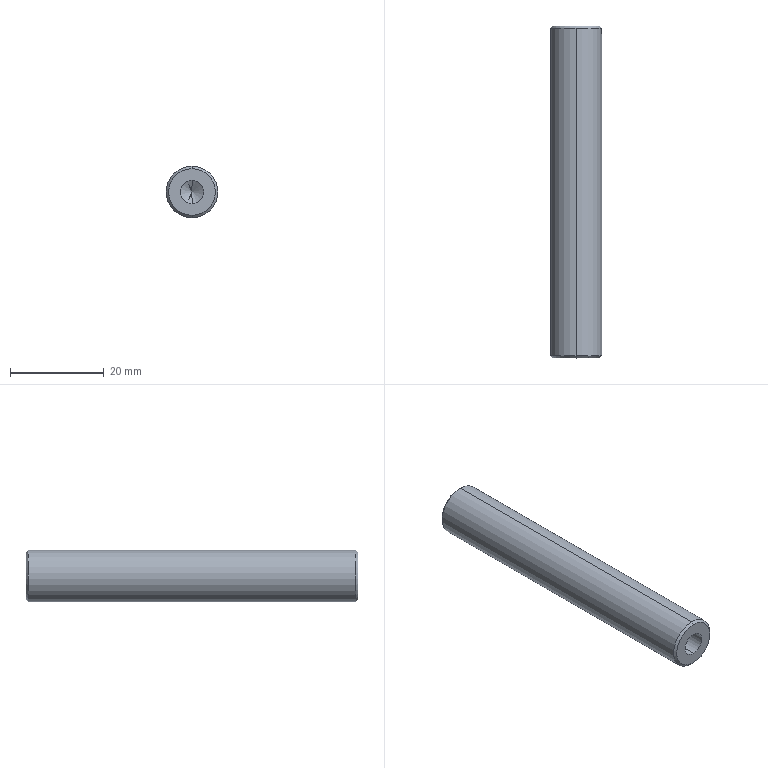Part | STEP file | 1105-104P043 | 1 solid | 16 faces | box 11 x 71 x 11 mm | volume 6130 mm3 | cone 8 | cylinder 6 | plane 2 | commonest cylinder face diameters 5 x4 11 x2
STEP:
#1=CARTESIAN_POINT('',(0.,0.,-5.));
#2=VERTEX_POINT('',#1);
#3=CARTESIAN_POINT('',(0.,0.,5.));
#4=VERTEX_POINT('',#3);
#5=CARTESIAN_POINT('',(0.,0.,0.));
#6=DIRECTION('',(0.,-1.,0.));
#7=DIRECTION('',(0.,0.,1.));
#8=AXIS2_PLACEMENT_3D('',#5,#6,#7);
#9=CIRCLE('',#8,5.);
#10=EDGE_CURVE('',#2,#4,#9,.T.);
#11=ORIENTED_EDGE('',*,*,#10,.F.);
#12=CARTESIAN_POINT('',(0.,0.5,-5.5));
#13=VERTEX_POINT('',#12);
#14=CARTESIAN_POINT('',(0.,0.5,-5.5));
#15=DIRECTION('',(0.,0.7071,-0.7071));
#16=VECTOR('',#15,1000.);
#17=LINE('',#14,#16);
#18=EDGE_CURVE('',#2,#13,#17,.T.);
#19=ORIENTED_EDGE('',*,*,#18,.T.);
#20=CARTESIAN_POINT('',(0.,0.5,5.5));
#21=VERTEX_POINT('',#20);
#22=CARTESIAN_POINT('',(0.,0.5,0.));
#23=DIRECTION('',(0.,1.,0.));
#24=DIRECTION('',(0.,0.,1.));
#25=AXIS2_PLACEMENT_3D('',#22,#23,#24);
#26=CIRCLE('',#25,5.5);
#27=EDGE_CURVE('',#21,#13,#26,.T.);
#28=ORIENTED_EDGE('',*,*,#27,.F.);
#29=CARTESIAN_POINT('',(0.,0.5,5.5));
#30=DIRECTION('',(0.,0.7071,0.7071));
#31=VECTOR('',#30,1000.);
#32=LINE('',#29,#31);
#33=EDGE_CURVE('',#4,#21,#32,.T.);
#34=ORIENTED_EDGE('',*,*,#33,.F.);
#35=EDGE_LOOP('',(#11,#19,#28,#34));
#36=FACE_OUTER_BOUND('',#35,.T.);
#37=CARTESIAN_POINT('',(0.,0.5,0.));
#38=DIRECTION('',(0.,1.,0.));
#39=DIRECTION('',(0.,0.,1.));
#40=AXIS2_PLACEMENT_3D('',#37,#38,#39);
#41=CONICAL_SURFACE('',#40,5.5,0.7854);
#42=ADVANCED_FACE('',(#36),#41,.T.);
#43=CARTESIAN_POINT('',(0.,71.,5.));
#44=VERTEX_POINT('',#43);
#45=CARTESIAN_POINT('',(0.,71.,-5.));
#46=VERTEX_POINT('',#45);
#47=CARTESIAN_POINT('',(0.,71.,0.));
#48=DIRECTION('',(0.,1.,0.));
#49=DIRECTION('',(0.,0.,1.));
#50=AXIS2_PLACEMENT_3D('',#47,#48,#49);
#51=CIRCLE('',#50,5.);
#52=EDGE_CURVE('',#44,#46,#51,.T.);
#53=ORIENTED_EDGE('',*,*,#52,.F.);
#54=CARTESIAN_POINT('',(0.,70.5,5.5));
#55=VERTEX_POINT('',#54);
#56=CARTESIAN_POINT('',(0.,71.,5.));
#57=DIRECTION('',(0.,-0.7071,0.7071));
#58=VECTOR('',#57,1000.);
#59=LINE('',#56,#58);
#60=EDGE_CURVE('',#44,#55,#59,.T.);
#61=ORIENTED_EDGE('',*,*,#60,.T.);
#62=CARTESIAN_POINT('',(0.,70.5,-5.5));
#63=VERTEX_POINT('',#62);
#64=CARTESIAN_POINT('',(0.,70.5,0.));
#65=DIRECTION('',(0.,-1.,0.));
#66=DIRECTION('',(0.,0.,1.));
#67=AXIS2_PLACEMENT_3D('',#64,#65,#66);
#68=CIRCLE('',#67,5.5);
#69=EDGE_CURVE('',#63,#55,#68,.T.);
#70=ORIENTED_EDGE('',*,*,#69,.F.);
#71=CARTESIAN_POINT('',(0.,71.,-5.));
#72=DIRECTION('',(0.,-0.7071,-0.7071));
#73=VECTOR('',#72,1000.);
#74=LINE('',#71,#73);
#75=EDGE_CURVE('',#46,#63,#74,.T.);
#76=ORIENTED_EDGE('',*,*,#75,.F.);
#77=EDGE_LOOP('',(#53,#61,#70,#76));
#78=FACE_OUTER_BOUND('',#77,.T.);
#79=CARTESIAN_POINT('',(0.,71.,0.));
#80=DIRECTION('',(0.,-1.,0.));
#81=DIRECTION('',(0.,0.,-1.));
#82=AXIS2_PLACEMENT_3D('',#79,#80,#81);
#83=CONICAL_SURFACE('',#82,5.,0.7854);
#84=ADVANCED_FACE('',(#78),#83,.T.);
#85=CARTESIAN_POINT('',(0.,15.,2.5));
#86=VERTEX_POINT('',#85);
#87=CARTESIAN_POINT('',(0.,15.,-2.5));
#88=VERTEX_POINT('',#87);
#89=CARTESIAN_POINT('',(0.,15.,0.));
#90=DIRECTION('',(0.,-1.,0.));
#91=DIRECTION('',(0.,0.,-1.));
#92=AXIS2_PLACEMENT_3D('',#89,#90,#91);
#93=CIRCLE('',#92,2.5);
#94=EDGE_CURVE('',#86,#88,#93,.T.);
#95=ORIENTED_EDGE('',*,*,#94,.F.);
#96=CARTESIAN_POINT('',(0.,0.,2.5));
#97=VERTEX_POINT('',#96);
#98=CARTESIAN_POINT('',(0.,0.,2.5));
#99=DIRECTION('',(0.,-1.,0.));
#100=VECTOR('',#99,1000.);
#101=LINE('',#98,#100);
#102=EDGE_CURVE('',#86,#97,#101,.T.);
#103=ORIENTED_EDGE('',*,*,#102,.T.);
#104=CARTESIAN_POINT('',(0.,0.,-2.5));
#105=VERTEX_POINT('',#104);
#106=CARTESIAN_POINT('',(0.,0.,0.));
#107=DIRECTION('',(0.,-1.,0.));
#108=DIRECTION('',(0.,0.,-1.));
#109=AXIS2_PLACEMENT_3D('',#106,#107,#108);
#110=CIRCLE('',#109,2.5);
#111=EDGE_CURVE('',#97,#105,#110,.T.);
#112=ORIENTED_EDGE('',*,*,#111,.T.);
#113=CARTESIAN_POINT('',(0.,0.,-2.5));
#114=DIRECTION('',(0.,-1.,0.));
#115=VECTOR('',#114,1000.);
#116=LINE('',#113,#115);
#117=EDGE_CURVE('',#88,#105,#116,.T.);
#118=ORIENTED_EDGE('',*,*,#117,.F.);
#119=EDGE_LOOP('',(#95,#103,#112,#118));
#120=FACE_OUTER_BOUND('',#119,.T.);
#121=CARTESIAN_POINT('',(0.,0.,0.));
#122=DIRECTION('',(0.,-1.,0.));
#123=DIRECTION('',(0.,0.,-1.));
#124=AXIS2_PLACEMENT_3D('',#121,#122,#123);
#125=CYLINDRICAL_SURFACE('',#124,2.5);
#126=ADVANCED_FACE('',(#120),#125,.F.);
#127=CARTESIAN_POINT('',(0.,16.502,0.));
#128=VERTEX_POINT('',#127);
#129=CARTESIAN_POINT('',(0.,15.,-2.5));
#130=DIRECTION('',(0.,-0.515,-0.8572));
#131=VECTOR('',#130,1000.);
#132=LINE('',#129,#131);
#133=EDGE_CURVE('',#128,#88,#132,.T.);
#134=ORIENTED_EDGE('',*,*,#133,.F.);
#135=CARTESIAN_POINT('',(0.,15.,2.5));
#136=DIRECTION('',(0.,-0.515,0.8572));
#137=VECTOR('',#136,1000.);
#138=LINE('',#135,#137);
#139=EDGE_CURVE('',#128,#86,#138,.T.);
#140=ORIENTED_EDGE('',*,*,#139,.T.);
#141=ORIENTED_EDGE('',*,*,#94,.T.);
#142=EDGE_LOOP('',(#134,#140,#141));
#143=FACE_OUTER_BOUND('',#142,.T.);
#144=CARTESIAN_POINT('',(0.,15.,0.));
#145=DIRECTION('',(0.,-1.,0.));
#146=DIRECTION('',(0.,0.,-1.));
#147=AXIS2_PLACEMENT_3D('',#144,#145,#146);
#148=CONICAL_SURFACE('',#147,2.5,1.03);
#149=ADVANCED_FACE('',(#143),#148,.F.);
#150=CARTESIAN_POINT('',(0.,56.,-2.5));
#151=VERTEX_POINT('',#150);
#152=CARTESIAN_POINT('',(0.,56.,2.5));
#153=VERTEX_POINT('',#152);
#154=CARTESIAN_POINT('',(0.,56.,0.));
#155=DIRECTION('',(0.,1.,0.));
#156=DIRECTION('',(0.,0.,1.));
#157=AXIS2_PLACEMENT_3D('',#154,#155,#156);
#158=CIRCLE('',#157,2.5);
#159=EDGE_CURVE('',#151,#153,#158,.T.);
#160=ORIENTED_EDGE('',*,*,#159,.F.);
#161=CARTESIAN_POINT('',(0.,71.,-2.5));
#162=VERTEX_POINT('',#161);
#163=CARTESIAN_POINT('',(0.,71.,-2.5));
#164=DIRECTION('',(0.,1.,0.));
#165=VECTOR('',#164,1000.);
#166=LINE('',#163,#165);
#167=EDGE_CURVE('',#151,#162,#166,.T.);
#168=ORIENTED_EDGE('',*,*,#167,.T.);
#169=CARTESIAN_POINT('',(0.,71.,2.5));
#170=VERTEX_POINT('',#169);
#171=CARTESIAN_POINT('',(0.,71.,0.));
#172=DIRECTION('',(0.,1.,0.));
#173=DIRECTION('',(0.,0.,1.));
#174=AXIS2_PLACEMENT_3D('',#171,#172,#173);
#175=CIRCLE('',#174,2.5);
#176=EDGE_CURVE('',#162,#170,#175,.T.);
#177=ORIENTED_EDGE('',*,*,#176,.T.);
#178=CARTESIAN_POINT('',(0.,71.,2.5));
#179=DIRECTION('',(0.,1.,0.));
#180=VECTOR('',#179,1000.);
#181=LINE('',#178,#180);
#182=EDGE_CURVE('',#153,#170,#181,.T.);
#183=ORIENTED_EDGE('',*,*,#182,.F.);
#184=EDGE_LOOP('',(#160,#168,#177,#183));
#185=FACE_OUTER_BOUND('',#184,.T.);
#186=CARTESIAN_POINT('',(0.,71.,0.));
#187=DIRECTION('',(0.,1.,0.));
#188=DIRECTION('',(0.,0.,1.));
#189=AXIS2_PLACEMENT_3D('',#186,#187,#188);
#190=CYLINDRICAL_SURFACE('',#189,2.5);
#191=ADVANCED_FACE('',(#185),#190,.F.);
#192=CARTESIAN_POINT('',(0.,54.498,0.));
#193=VERTEX_POINT('',#192);
#194=CARTESIAN_POINT('',(0.,56.,2.5));
#195=DIRECTION('',(0.,0.515,0.8572));
#196=VECTOR('',#195,1000.);
#197=LINE('',#194,#196);
#198=EDGE_CURVE('',#193,#153,#197,.T.);
#199=ORIENTED_EDGE('',*,*,#198,.F.);
#200=CARTESIAN_POINT('',(0.,56.,-2.5));
#201=DIRECTION('',(0.,0.515,-0.8572));
#202=VECTOR('',#201,1000.);
#203=LINE('',#200,#202);
#204=EDGE_CURVE('',#193,#151,#203,.T.);
#205=ORIENTED_EDGE('',*,*,#204,.T.);
#206=ORIENTED_EDGE('',*,*,#159,.T.);
#207=EDGE_LOOP('',(#199,#205,#206));
#208=FACE_OUTER_BOUND('',#207,.T.);
#209=CARTESIAN_POINT('',(0.,56.,0.));
#210=DIRECTION('',(0.,1.,0.));
#211=DIRECTION('',(0.,0.,1.));
#212=AXIS2_PLACEMENT_3D('',#209,#210,#211);
#213=CONICAL_SURFACE('',#212,2.5,1.03);
#214=ADVANCED_FACE('',(#208),#213,.F.);
#215=ORIENTED_EDGE('',*,*,#69,.T.);
#216=CARTESIAN_POINT('',(0.,71.,5.5));
#217=DIRECTION('',(0.,-1.,0.));
#218=VECTOR('',#217,1000.);
#219=LINE('',#216,#218);
#220=EDGE_CURVE('',#55,#21,#219,.T.);
#221=ORIENTED_EDGE('',*,*,#220,.T.);
#222=ORIENTED_EDGE('',*,*,#27,.T.);
#223=CARTESIAN_POINT('',(0.,71.,-5.5));
#224=DIRECTION('',(0.,-1.,0.));
#225=VECTOR('',#224,1000.);
#226=LINE('',#223,#225);
#227=EDGE_CURVE('',#63,#13,#226,.T.);
#228=ORIENTED_EDGE('',*,*,#227,.F.);
#229=EDGE_LOOP('',(#215,#221,#222,#228));
#230=FACE_OUTER_BOUND('',#229,.T.);
#231=CARTESIAN_POINT('',(0.,71.,0.));
#232=DIRECTION('',(0.,-1.,0.));
#233=DIRECTION('',(0.,0.,-1.));
#234=AXIS2_PLACEMENT_3D('',#231,#232,#233);
#235=CYLINDRICAL_SURFACE('',#234,5.5);
#236=ADVANCED_FACE('',(#230),#235,.T.);
#237=ORIENTED_EDGE('',*,*,#220,.F.);
#238=CARTESIAN_POINT('',(0.,70.5,0.));
#239=DIRECTION('',(0.,-1.,0.));
#240=DIRECTION('',(0.,0.,1.));
#241=AXIS2_PLACEMENT_3D('',#238,#239,#240);
#242=CIRCLE('',#241,5.5);
#243=EDGE_CURVE('',#55,#63,#242,.T.);
#244=ORIENTED_EDGE('',*,*,#243,.T.);
#245=ORIENTED_EDGE('',*,*,#227,.T.);
#246=CARTESIAN_POINT('',(0.,0.5,0.));
#247=DIRECTION('',(0.,1.,0.));
#248=DIRECTION('',(0.,0.,1.));
#249=AXIS2_PLACEMENT_3D('',#246,#247,#248);
#250=CIRCLE('',#249,5.5);
#251=EDGE_CURVE('',#13,#21,#250,.T.);
#252=ORIENTED_EDGE('',*,*,#251,.T.);
#253=EDGE_LOOP('',(#237,#244,#245,#252));
#254=FACE_OUTER_BOUND('',#253,.T.);
#255=CARTESIAN_POINT('',(0.,71.,0.));
#256=DIRECTION('',(0.,-1.,0.));
#257=DIRECTION('',(0.,0.,-1.));
#258=AXIS2_PLACEMENT_3D('',#255,#256,#257);
#259=CYLINDRICAL_SURFACE('',#258,5.5);
#260=ADVANCED_FACE('',(#254),#259,.T.);
#261=CARTESIAN_POINT('',(0.,71.,0.));
#262=DIRECTION('',(0.,1.,0.));
#263=DIRECTION('',(0.,0.,1.));
#264=AXIS2_PLACEMENT_3D('',#261,#262,#263);
#265=CIRCLE('',#264,5.);
#266=EDGE_CURVE('',#46,#44,#265,.T.);
#267=ORIENTED_EDGE('',*,*,#266,.T.);
#268=ORIENTED_EDGE('',*,*,#52,.T.);
#269=EDGE_LOOP('',(#267,#268));
#270=FACE_OUTER_BOUND('',#269,.T.);
#271=CARTESIAN_POINT('',(0.,71.,0.));
#272=DIRECTION('',(0.,1.,0.));
#273=DIRECTION('',(0.,0.,1.));
#274=AXIS2_PLACEMENT_3D('',#271,#272,#273);
#275=CIRCLE('',#274,2.5);
#276=EDGE_CURVE('',#170,#162,#275,.T.);
#277=ORIENTED_EDGE('',*,*,#276,.F.);
#278=ORIENTED_EDGE('',*,*,#176,.F.);
#279=EDGE_LOOP('',(#277,#278));
#280=FACE_BOUND('',#279,.T.);
#281=CARTESIAN_POINT('',(0.,71.,0.));
#282=DIRECTION('',(0.,1.,0.));
#283=DIRECTION('',(0.,0.,1.));
#284=AXIS2_PLACEMENT_3D('',#281,#282,#283);
#285=PLANE('',#284);
#286=ADVANCED_FACE('',(#270,#280),#285,.T.);
#287=CARTESIAN_POINT('',(0.,0.,0.));
#288=DIRECTION('',(0.,-1.,0.));
#289=DIRECTION('',(0.,0.,1.));
#290=AXIS2_PLACEMENT_3D('',#287,#288,#289);
#291=CIRCLE('',#290,5.);
#292=EDGE_CURVE('',#4,#2,#291,.T.);
#293=ORIENTED_EDGE('',*,*,#292,.T.);
#294=ORIENTED_EDGE('',*,*,#10,.T.);
#295=EDGE_LOOP('',(#293,#294));
#296=FACE_OUTER_BOUND('',#295,.T.);
#297=CARTESIAN_POINT('',(0.,0.,0.));
#298=DIRECTION('',(0.,-1.,0.));
#299=DIRECTION('',(0.,0.,-1.));
#300=AXIS2_PLACEMENT_3D('',#297,#298,#299);
#301=CIRCLE('',#300,2.5);
#302=EDGE_CURVE('',#105,#97,#301,.T.);
#303=ORIENTED_EDGE('',*,*,#302,.F.);
#304=ORIENTED_EDGE('',*,*,#111,.F.);
#305=EDGE_LOOP('',(#303,#304));
#306=FACE_BOUND('',#305,.T.);
#307=CARTESIAN_POINT('',(0.,0.,0.));
#308=DIRECTION('',(0.,1.,0.));
#309=DIRECTION('',(0.,0.,1.));
#310=AXIS2_PLACEMENT_3D('',#307,#308,#309);
#311=PLANE('',#310);
#312=ADVANCED_FACE('',(#296,#306),#311,.F.);
#313=ORIENTED_EDGE('',*,*,#204,.F.);
#314=ORIENTED_EDGE('',*,*,#198,.T.);
#315=CARTESIAN_POINT('',(0.,56.,0.));
#316=DIRECTION('',(0.,1.,0.));
#317=DIRECTION('',(0.,0.,1.));
#318=AXIS2_PLACEMENT_3D('',#315,#316,#317);
#319=CIRCLE('',#318,2.5);
#320=EDGE_CURVE('',#153,#151,#319,.T.);
#321=ORIENTED_EDGE('',*,*,#320,.T.);
#322=EDGE_LOOP('',(#313,#314,#321));
#323=FACE_OUTER_BOUND('',#322,.T.);
#324=CARTESIAN_POINT('',(0.,56.,0.));
#325=DIRECTION('',(0.,1.,0.));
#326=DIRECTION('',(0.,0.,1.));
#327=AXIS2_PLACEMENT_3D('',#324,#325,#326);
#328=CONICAL_SURFACE('',#327,2.5,1.03);
#329=ADVANCED_FACE('',(#323),#328,.F.);
#330=ORIENTED_EDGE('',*,*,#167,.F.);
#331=ORIENTED_EDGE('',*,*,#320,.F.);
#332=ORIENTED_EDGE('',*,*,#182,.T.);
#333=ORIENTED_EDGE('',*,*,#276,.T.);
#334=EDGE_LOOP('',(#330,#331,#332,#333));
#335=FACE_OUTER_BOUND('',#334,.T.);
#336=CARTESIAN_POINT('',(0.,71.,0.));
#337=DIRECTION('',(0.,1.,0.));
#338=DIRECTION('',(0.,0.,1.));
#339=AXIS2_PLACEMENT_3D('',#336,#337,#338);
#340=CYLINDRICAL_SURFACE('',#339,2.5);
#341=ADVANCED_FACE('',(#335),#340,.F.);
#342=ORIENTED_EDGE('',*,*,#139,.F.);
#343=ORIENTED_EDGE('',*,*,#133,.T.);
#344=CARTESIAN_POINT('',(0.,15.,0.));
#345=DIRECTION('',(0.,-1.,0.));
#346=DIRECTION('',(0.,0.,-1.));
#347=AXIS2_PLACEMENT_3D('',#344,#345,#346);
#348=CIRCLE('',#347,2.5);
#349=EDGE_CURVE('',#88,#86,#348,.T.);
#350=ORIENTED_EDGE('',*,*,#349,.T.);
#351=EDGE_LOOP('',(#342,#343,#350));
#352=FACE_OUTER_BOUND('',#351,.T.);
#353=CARTESIAN_POINT('',(0.,15.,0.));
#354=DIRECTION('',(0.,-1.,0.));
#355=DIRECTION('',(0.,0.,-1.));
#356=AXIS2_PLACEMENT_3D('',#353,#354,#355);
#357=CONICAL_SURFACE('',#356,2.5,1.03);
#358=ADVANCED_FACE('',(#352),#357,.F.);
#359=ORIENTED_EDGE('',*,*,#102,.F.);
#360=ORIENTED_EDGE('',*,*,#349,.F.);
#361=ORIENTED_EDGE('',*,*,#117,.T.);
#362=ORIENTED_EDGE('',*,*,#302,.T.);
#363=EDGE_LOOP('',(#359,#360,#361,#362));
#364=FACE_OUTER_BOUND('',#363,.T.);
#365=CARTESIAN_POINT('',(0.,0.,0.));
#366=DIRECTION('',(0.,-1.,0.));
#367=DIRECTION('',(0.,0.,-1.));
#368=AXIS2_PLACEMENT_3D('',#365,#366,#367);
#369=CYLINDRICAL_SURFACE('',#368,2.5);
#370=ADVANCED_FACE('',(#364),#369,.F.);
#371=ORIENTED_EDGE('',*,*,#60,.F.);
#372=ORIENTED_EDGE('',*,*,#266,.F.);
#373=ORIENTED_EDGE('',*,*,#75,.T.);
#374=ORIENTED_EDGE('',*,*,#243,.F.);
#375=EDGE_LOOP('',(#371,#372,#373,#374));
#376=FACE_OUTER_BOUND('',#375,.T.);
#377=CARTESIAN_POINT('',(0.,71.,0.));
#378=DIRECTION('',(0.,-1.,0.));
#379=DIRECTION('',(0.,0.,-1.));
#380=AXIS2_PLACEMENT_3D('',#377,#378,#379);
#381=CONICAL_SURFACE('',#380,5.,0.7854);
#382=ADVANCED_FACE('',(#376),#381,.T.);
#383=ORIENTED_EDGE('',*,*,#18,.F.);
#384=ORIENTED_EDGE('',*,*,#292,.F.);
#385=ORIENTED_EDGE('',*,*,#33,.T.);
#386=ORIENTED_EDGE('',*,*,#251,.F.);
#387=EDGE_LOOP('',(#383,#384,#385,#386));
#388=FACE_OUTER_BOUND('',#387,.T.);
#389=CARTESIAN_POINT('',(0.,0.5,0.));
#390=DIRECTION('',(0.,1.,0.));
#391=DIRECTION('',(0.,0.,1.));
#392=AXIS2_PLACEMENT_3D('',#389,#390,#391);
#393=CONICAL_SURFACE('',#392,5.5,0.7854);
#394=ADVANCED_FACE('',(#388),#393,.T.);
#395=CLOSED_SHELL('',(#42,#84,#126,#149,#191,#214,#236,#260,#286,#312,#329,#341,#358,#370,#382,#394));
#396=MANIFOLD_SOLID_BREP('',#395);
#397=CARTESIAN_POINT('',(0.,0.,0.));
#398=DIRECTION('',(0.,0.,1.));
#399=DIRECTION('',(1.,0.,0.));
#400=AXIS2_PLACEMENT_3D('',#397,#398,#399);
#401=(LENGTH_UNIT()NAMED_UNIT(*)SI_UNIT(.MILLI.,.METRE.));
#402=UNCERTAINTY_MEASURE_WITH_UNIT(LENGTH_MEASURE(0.00001),#401,'','');
#403=(NAMED_UNIT(*)PLANE_ANGLE_UNIT()SI_UNIT($,.RADIAN.));
#404=(NAMED_UNIT(*)SI_UNIT($,.STERADIAN.)SOLID_ANGLE_UNIT());
#405=(GEOMETRIC_REPRESENTATION_CONTEXT(3)GLOBAL_UNCERTAINTY_ASSIGNED_CONTEXT((#402))GLOBAL_UNIT_ASSIGNED_CONTEXT((#401,#403,#404))REPRESENTATION_CONTEXT('',''));
#406=ADVANCED_BREP_SHAPE_REPRESENTATION('',(#396,#400),#405);